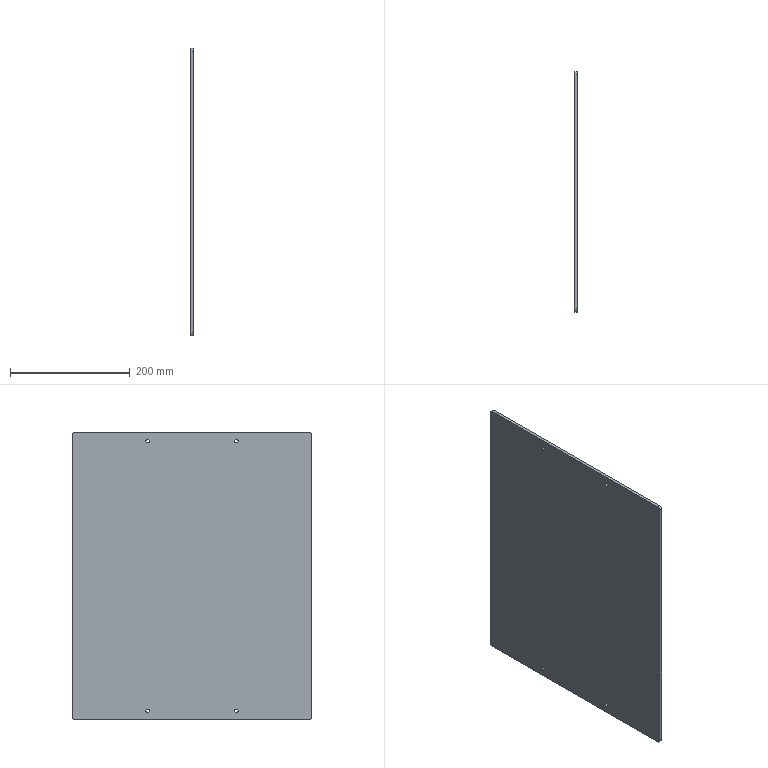Part | SolidWorks | features Extrusion 1, Fillet 1, ICE 1 | 1 solid | 18 faces | box 5 x 400 x 480 mm | volume 959327 mm3 | cylinder 12 | plane 6 | commonest cylinder face diameters 6 x8 10 x4
STEP:
#1=CARTESIAN_POINT('',(0.,-74.,-222.));
#2=VERTEX_POINT('',#1);
#3=CARTESIAN_POINT('',(0.,-74.,-228.));
#4=VERTEX_POINT('',#3);
#5=CARTESIAN_POINT('',(0.,-74.,-225.));
#6=DIRECTION('',(1.,0.,0.));
#7=DIRECTION('',(0.,0.,-1.));
#8=AXIS2_PLACEMENT_3D('',#5,#6,#7);
#9=CIRCLE('',#8,3.);
#10=EDGE_CURVE('',#2,#4,#9,.T.);
#11=ORIENTED_EDGE('',*,*,#10,.F.);
#12=CARTESIAN_POINT('',(5.,-74.,-222.));
#13=VERTEX_POINT('',#12);
#14=CARTESIAN_POINT('',(0.,-74.,-222.));
#15=DIRECTION('',(1.,0.,0.));
#16=VECTOR('',#15,1000.);
#17=LINE('',#14,#16);
#18=EDGE_CURVE('',#2,#13,#17,.T.);
#19=ORIENTED_EDGE('',*,*,#18,.T.);
#20=CARTESIAN_POINT('',(5.,-74.,-228.));
#21=VERTEX_POINT('',#20);
#22=CARTESIAN_POINT('',(5.,-74.,-225.));
#23=DIRECTION('',(1.,0.,0.));
#24=DIRECTION('',(0.,0.,-1.));
#25=AXIS2_PLACEMENT_3D('',#22,#23,#24);
#26=CIRCLE('',#25,3.);
#27=EDGE_CURVE('',#13,#21,#26,.T.);
#28=ORIENTED_EDGE('',*,*,#27,.T.);
#29=CARTESIAN_POINT('',(0.,-74.,-228.));
#30=DIRECTION('',(1.,0.,0.));
#31=VECTOR('',#30,1000.);
#32=LINE('',#29,#31);
#33=EDGE_CURVE('',#4,#21,#32,.T.);
#34=ORIENTED_EDGE('',*,*,#33,.F.);
#35=EDGE_LOOP('',(#11,#19,#28,#34));
#36=FACE_OUTER_BOUND('',#35,.T.);
#37=CARTESIAN_POINT('',(0.,-74.,-225.));
#38=DIRECTION('',(1.,0.,0.));
#39=DIRECTION('',(0.,0.,-1.));
#40=AXIS2_PLACEMENT_3D('',#37,#38,#39);
#41=CYLINDRICAL_SURFACE('',#40,3.);
#42=ADVANCED_FACE('',(#36),#41,.F.);
#43=CARTESIAN_POINT('',(0.,-74.,228.));
#44=VERTEX_POINT('',#43);
#45=CARTESIAN_POINT('',(0.,-74.,222.));
#46=VERTEX_POINT('',#45);
#47=CARTESIAN_POINT('',(0.,-74.,225.));
#48=DIRECTION('',(1.,0.,0.));
#49=DIRECTION('',(0.,0.,-1.));
#50=AXIS2_PLACEMENT_3D('',#47,#48,#49);
#51=CIRCLE('',#50,3.);
#52=EDGE_CURVE('',#44,#46,#51,.T.);
#53=ORIENTED_EDGE('',*,*,#52,.F.);
#54=CARTESIAN_POINT('',(5.,-74.,228.));
#55=VERTEX_POINT('',#54);
#56=CARTESIAN_POINT('',(0.,-74.,228.));
#57=DIRECTION('',(1.,0.,0.));
#58=VECTOR('',#57,1000.);
#59=LINE('',#56,#58);
#60=EDGE_CURVE('',#44,#55,#59,.T.);
#61=ORIENTED_EDGE('',*,*,#60,.T.);
#62=CARTESIAN_POINT('',(5.,-74.,222.));
#63=VERTEX_POINT('',#62);
#64=CARTESIAN_POINT('',(5.,-74.,225.));
#65=DIRECTION('',(1.,0.,0.));
#66=DIRECTION('',(0.,0.,-1.));
#67=AXIS2_PLACEMENT_3D('',#64,#65,#66);
#68=CIRCLE('',#67,3.);
#69=EDGE_CURVE('',#55,#63,#68,.T.);
#70=ORIENTED_EDGE('',*,*,#69,.T.);
#71=CARTESIAN_POINT('',(0.,-74.,222.));
#72=DIRECTION('',(1.,0.,0.));
#73=VECTOR('',#72,1000.);
#74=LINE('',#71,#73);
#75=EDGE_CURVE('',#46,#63,#74,.T.);
#76=ORIENTED_EDGE('',*,*,#75,.F.);
#77=EDGE_LOOP('',(#53,#61,#70,#76));
#78=FACE_OUTER_BOUND('',#77,.T.);
#79=CARTESIAN_POINT('',(0.,-74.,225.));
#80=DIRECTION('',(1.,0.,0.));
#81=DIRECTION('',(0.,0.,-1.));
#82=AXIS2_PLACEMENT_3D('',#79,#80,#81);
#83=CYLINDRICAL_SURFACE('',#82,3.);
#84=ADVANCED_FACE('',(#78),#83,.F.);
#85=CARTESIAN_POINT('',(0.,74.,-222.));
#86=VERTEX_POINT('',#85);
#87=CARTESIAN_POINT('',(0.,74.,-228.));
#88=VERTEX_POINT('',#87);
#89=CARTESIAN_POINT('',(0.,74.,-225.));
#90=DIRECTION('',(1.,0.,0.));
#91=DIRECTION('',(0.,0.,-1.));
#92=AXIS2_PLACEMENT_3D('',#89,#90,#91);
#93=CIRCLE('',#92,3.);
#94=EDGE_CURVE('',#86,#88,#93,.T.);
#95=ORIENTED_EDGE('',*,*,#94,.F.);
#96=CARTESIAN_POINT('',(5.,74.,-222.));
#97=VERTEX_POINT('',#96);
#98=CARTESIAN_POINT('',(0.,74.,-222.));
#99=DIRECTION('',(1.,0.,0.));
#100=VECTOR('',#99,1000.);
#101=LINE('',#98,#100);
#102=EDGE_CURVE('',#86,#97,#101,.T.);
#103=ORIENTED_EDGE('',*,*,#102,.T.);
#104=CARTESIAN_POINT('',(5.,74.,-228.));
#105=VERTEX_POINT('',#104);
#106=CARTESIAN_POINT('',(5.,74.,-225.));
#107=DIRECTION('',(1.,0.,0.));
#108=DIRECTION('',(0.,0.,-1.));
#109=AXIS2_PLACEMENT_3D('',#106,#107,#108);
#110=CIRCLE('',#109,3.);
#111=EDGE_CURVE('',#97,#105,#110,.T.);
#112=ORIENTED_EDGE('',*,*,#111,.T.);
#113=CARTESIAN_POINT('',(0.,74.,-228.));
#114=DIRECTION('',(1.,0.,0.));
#115=VECTOR('',#114,1000.);
#116=LINE('',#113,#115);
#117=EDGE_CURVE('',#88,#105,#116,.T.);
#118=ORIENTED_EDGE('',*,*,#117,.F.);
#119=EDGE_LOOP('',(#95,#103,#112,#118));
#120=FACE_OUTER_BOUND('',#119,.T.);
#121=CARTESIAN_POINT('',(0.,74.,-225.));
#122=DIRECTION('',(1.,0.,0.));
#123=DIRECTION('',(0.,0.,-1.));
#124=AXIS2_PLACEMENT_3D('',#121,#122,#123);
#125=CYLINDRICAL_SURFACE('',#124,3.);
#126=ADVANCED_FACE('',(#120),#125,.F.);
#127=CARTESIAN_POINT('',(0.,74.,228.));
#128=VERTEX_POINT('',#127);
#129=CARTESIAN_POINT('',(0.,74.,222.));
#130=VERTEX_POINT('',#129);
#131=CARTESIAN_POINT('',(0.,74.,225.));
#132=DIRECTION('',(1.,0.,0.));
#133=DIRECTION('',(0.,0.,-1.));
#134=AXIS2_PLACEMENT_3D('',#131,#132,#133);
#135=CIRCLE('',#134,3.);
#136=EDGE_CURVE('',#128,#130,#135,.T.);
#137=ORIENTED_EDGE('',*,*,#136,.F.);
#138=CARTESIAN_POINT('',(5.,74.,228.));
#139=VERTEX_POINT('',#138);
#140=CARTESIAN_POINT('',(0.,74.,228.));
#141=DIRECTION('',(1.,0.,0.));
#142=VECTOR('',#141,1000.);
#143=LINE('',#140,#142);
#144=EDGE_CURVE('',#128,#139,#143,.T.);
#145=ORIENTED_EDGE('',*,*,#144,.T.);
#146=CARTESIAN_POINT('',(5.,74.,222.));
#147=VERTEX_POINT('',#146);
#148=CARTESIAN_POINT('',(5.,74.,225.));
#149=DIRECTION('',(1.,0.,0.));
#150=DIRECTION('',(0.,0.,-1.));
#151=AXIS2_PLACEMENT_3D('',#148,#149,#150);
#152=CIRCLE('',#151,3.);
#153=EDGE_CURVE('',#139,#147,#152,.T.);
#154=ORIENTED_EDGE('',*,*,#153,.T.);
#155=CARTESIAN_POINT('',(0.,74.,222.));
#156=DIRECTION('',(1.,0.,0.));
#157=VECTOR('',#156,1000.);
#158=LINE('',#155,#157);
#159=EDGE_CURVE('',#130,#147,#158,.T.);
#160=ORIENTED_EDGE('',*,*,#159,.F.);
#161=EDGE_LOOP('',(#137,#145,#154,#160));
#162=FACE_OUTER_BOUND('',#161,.T.);
#163=CARTESIAN_POINT('',(0.,74.,225.));
#164=DIRECTION('',(1.,0.,0.));
#165=DIRECTION('',(0.,0.,-1.));
#166=AXIS2_PLACEMENT_3D('',#163,#164,#165);
#167=CYLINDRICAL_SURFACE('',#166,3.);
#168=ADVANCED_FACE('',(#162),#167,.F.);
#169=CARTESIAN_POINT('',(0.,195.,240.));
#170=VERTEX_POINT('',#169);
#171=CARTESIAN_POINT('',(0.,-195.,240.));
#172=VERTEX_POINT('',#171);
#173=CARTESIAN_POINT('',(0.,200.,240.));
#174=DIRECTION('',(0.,-1.,0.));
#175=VECTOR('',#174,1000.);
#176=LINE('',#173,#175);
#177=EDGE_CURVE('',#170,#172,#176,.T.);
#178=ORIENTED_EDGE('',*,*,#177,.T.);
#179=CARTESIAN_POINT('',(5.,-195.,240.));
#180=VERTEX_POINT('',#179);
#181=CARTESIAN_POINT('',(5.,-195.,240.));
#182=DIRECTION('',(1.,0.,0.));
#183=VECTOR('',#182,1000.);
#184=LINE('',#181,#183);
#185=EDGE_CURVE('',#172,#180,#184,.T.);
#186=ORIENTED_EDGE('',*,*,#185,.T.);
#187=CARTESIAN_POINT('',(5.,195.,240.));
#188=VERTEX_POINT('',#187);
#189=CARTESIAN_POINT('',(5.,200.,240.));
#190=DIRECTION('',(0.,-1.,0.));
#191=VECTOR('',#190,1000.);
#192=LINE('',#189,#191);
#193=EDGE_CURVE('',#188,#180,#192,.T.);
#194=ORIENTED_EDGE('',*,*,#193,.F.);
#195=CARTESIAN_POINT('',(5.,195.,240.));
#196=DIRECTION('',(-1.,0.,0.));
#197=VECTOR('',#196,1000.);
#198=LINE('',#195,#197);
#199=EDGE_CURVE('',#188,#170,#198,.T.);
#200=ORIENTED_EDGE('',*,*,#199,.T.);
#201=EDGE_LOOP('',(#178,#186,#194,#200));
#202=FACE_OUTER_BOUND('',#201,.T.);
#203=CARTESIAN_POINT('',(5.,200.,240.));
#204=DIRECTION('',(0.,0.,-1.));
#205=DIRECTION('',(-1.,0.,0.));
#206=AXIS2_PLACEMENT_3D('',#203,#204,#205);
#207=PLANE('',#206);
#208=ADVANCED_FACE('',(#202),#207,.F.);
#209=CARTESIAN_POINT('',(5.,-200.,235.));
#210=VERTEX_POINT('',#209);
#211=CARTESIAN_POINT('',(5.,-200.,-235.));
#212=VERTEX_POINT('',#211);
#213=CARTESIAN_POINT('',(5.,-200.,240.));
#214=DIRECTION('',(0.,0.,-1.));
#215=VECTOR('',#214,1000.);
#216=LINE('',#213,#215);
#217=EDGE_CURVE('',#210,#212,#216,.T.);
#218=ORIENTED_EDGE('',*,*,#217,.F.);
#219=CARTESIAN_POINT('',(0.,-200.,235.));
#220=VERTEX_POINT('',#219);
#221=CARTESIAN_POINT('',(5.,-200.,235.));
#222=DIRECTION('',(-1.,0.,0.));
#223=VECTOR('',#222,1000.);
#224=LINE('',#221,#223);
#225=EDGE_CURVE('',#210,#220,#224,.T.);
#226=ORIENTED_EDGE('',*,*,#225,.T.);
#227=CARTESIAN_POINT('',(0.,-200.,-235.));
#228=VERTEX_POINT('',#227);
#229=CARTESIAN_POINT('',(0.,-200.,240.));
#230=DIRECTION('',(0.,0.,-1.));
#231=VECTOR('',#230,1000.);
#232=LINE('',#229,#231);
#233=EDGE_CURVE('',#220,#228,#232,.T.);
#234=ORIENTED_EDGE('',*,*,#233,.T.);
#235=CARTESIAN_POINT('',(5.,-200.,-235.));
#236=DIRECTION('',(1.,0.,0.));
#237=VECTOR('',#236,1000.);
#238=LINE('',#235,#237);
#239=EDGE_CURVE('',#228,#212,#238,.T.);
#240=ORIENTED_EDGE('',*,*,#239,.T.);
#241=EDGE_LOOP('',(#218,#226,#234,#240));
#242=FACE_OUTER_BOUND('',#241,.T.);
#243=CARTESIAN_POINT('',(5.,-200.,240.));
#244=DIRECTION('',(0.,1.,0.));
#245=DIRECTION('',(0.,0.,1.));
#246=AXIS2_PLACEMENT_3D('',#243,#244,#245);
#247=PLANE('',#246);
#248=ADVANCED_FACE('',(#242),#247,.F.);
#249=CARTESIAN_POINT('',(5.,-195.,-240.));
#250=VERTEX_POINT('',#249);
#251=CARTESIAN_POINT('',(5.,195.,-240.));
#252=VERTEX_POINT('',#251);
#253=CARTESIAN_POINT('',(5.,200.,-240.));
#254=DIRECTION('',(0.,1.,0.));
#255=VECTOR('',#254,1000.);
#256=LINE('',#253,#255);
#257=EDGE_CURVE('',#250,#252,#256,.T.);
#258=ORIENTED_EDGE('',*,*,#257,.F.);
#259=CARTESIAN_POINT('',(0.,-195.,-240.));
#260=VERTEX_POINT('',#259);
#261=CARTESIAN_POINT('',(5.,-195.,-240.));
#262=DIRECTION('',(-1.,0.,0.));
#263=VECTOR('',#262,1000.);
#264=LINE('',#261,#263);
#265=EDGE_CURVE('',#250,#260,#264,.T.);
#266=ORIENTED_EDGE('',*,*,#265,.T.);
#267=CARTESIAN_POINT('',(0.,195.,-240.));
#268=VERTEX_POINT('',#267);
#269=CARTESIAN_POINT('',(0.,200.,-240.));
#270=DIRECTION('',(0.,1.,0.));
#271=VECTOR('',#270,1000.);
#272=LINE('',#269,#271);
#273=EDGE_CURVE('',#260,#268,#272,.T.);
#274=ORIENTED_EDGE('',*,*,#273,.T.);
#275=CARTESIAN_POINT('',(5.,195.,-240.));
#276=DIRECTION('',(1.,0.,0.));
#277=VECTOR('',#276,1000.);
#278=LINE('',#275,#277);
#279=EDGE_CURVE('',#268,#252,#278,.T.);
#280=ORIENTED_EDGE('',*,*,#279,.T.);
#281=EDGE_LOOP('',(#258,#266,#274,#280));
#282=FACE_OUTER_BOUND('',#281,.T.);
#283=CARTESIAN_POINT('',(5.,200.,-240.));
#284=DIRECTION('',(0.,0.,1.));
#285=DIRECTION('',(1.,0.,0.));
#286=AXIS2_PLACEMENT_3D('',#283,#284,#285);
#287=PLANE('',#286);
#288=ADVANCED_FACE('',(#282),#287,.F.);
#289=CARTESIAN_POINT('',(5.,200.,-235.));
#290=VERTEX_POINT('',#289);
#291=CARTESIAN_POINT('',(5.,200.,235.));
#292=VERTEX_POINT('',#291);
#293=CARTESIAN_POINT('',(5.,200.,240.));
#294=DIRECTION('',(0.,0.,1.));
#295=VECTOR('',#294,1000.);
#296=LINE('',#293,#295);
#297=EDGE_CURVE('',#290,#292,#296,.T.);
#298=ORIENTED_EDGE('',*,*,#297,.F.);
#299=CARTESIAN_POINT('',(0.,200.,-235.));
#300=VERTEX_POINT('',#299);
#301=CARTESIAN_POINT('',(5.,200.,-235.));
#302=DIRECTION('',(-1.,0.,0.));
#303=VECTOR('',#302,1000.);
#304=LINE('',#301,#303);
#305=EDGE_CURVE('',#290,#300,#304,.T.);
#306=ORIENTED_EDGE('',*,*,#305,.T.);
#307=CARTESIAN_POINT('',(0.,200.,235.));
#308=VERTEX_POINT('',#307);
#309=CARTESIAN_POINT('',(0.,200.,240.));
#310=DIRECTION('',(0.,0.,1.));
#311=VECTOR('',#310,1000.);
#312=LINE('',#309,#311);
#313=EDGE_CURVE('',#300,#308,#312,.T.);
#314=ORIENTED_EDGE('',*,*,#313,.T.);
#315=CARTESIAN_POINT('',(5.,200.,235.));
#316=DIRECTION('',(1.,0.,0.));
#317=VECTOR('',#316,1000.);
#318=LINE('',#315,#317);
#319=EDGE_CURVE('',#308,#292,#318,.T.);
#320=ORIENTED_EDGE('',*,*,#319,.T.);
#321=EDGE_LOOP('',(#298,#306,#314,#320));
#322=FACE_OUTER_BOUND('',#321,.T.);
#323=CARTESIAN_POINT('',(5.,200.,240.));
#324=DIRECTION('',(0.,-1.,0.));
#325=DIRECTION('',(0.,0.,-1.));
#326=AXIS2_PLACEMENT_3D('',#323,#324,#325);
#327=PLANE('',#326);
#328=ADVANCED_FACE('',(#322),#327,.F.);
#329=CARTESIAN_POINT('',(5.,-74.,-225.));
#330=DIRECTION('',(1.,0.,0.));
#331=DIRECTION('',(0.,0.,-1.));
#332=AXIS2_PLACEMENT_3D('',#329,#330,#331);
#333=CIRCLE('',#332,3.);
#334=EDGE_CURVE('',#21,#13,#333,.T.);
#335=ORIENTED_EDGE('',*,*,#334,.F.);
#336=ORIENTED_EDGE('',*,*,#27,.F.);
#337=EDGE_LOOP('',(#335,#336));
#338=FACE_BOUND('',#337,.T.);
#339=CARTESIAN_POINT('',(5.,-74.,225.));
#340=DIRECTION('',(1.,0.,0.));
#341=DIRECTION('',(0.,0.,-1.));
#342=AXIS2_PLACEMENT_3D('',#339,#340,#341);
#343=CIRCLE('',#342,3.);
#344=EDGE_CURVE('',#63,#55,#343,.T.);
#345=ORIENTED_EDGE('',*,*,#344,.F.);
#346=ORIENTED_EDGE('',*,*,#69,.F.);
#347=EDGE_LOOP('',(#345,#346));
#348=FACE_BOUND('',#347,.T.);
#349=CARTESIAN_POINT('',(5.,74.,-225.));
#350=DIRECTION('',(1.,0.,0.));
#351=DIRECTION('',(0.,0.,-1.));
#352=AXIS2_PLACEMENT_3D('',#349,#350,#351);
#353=CIRCLE('',#352,3.);
#354=EDGE_CURVE('',#105,#97,#353,.T.);
#355=ORIENTED_EDGE('',*,*,#354,.F.);
#356=ORIENTED_EDGE('',*,*,#111,.F.);
#357=EDGE_LOOP('',(#355,#356));
#358=FACE_BOUND('',#357,.T.);
#359=CARTESIAN_POINT('',(5.,74.,225.));
#360=DIRECTION('',(1.,0.,0.));
#361=DIRECTION('',(0.,0.,-1.));
#362=AXIS2_PLACEMENT_3D('',#359,#360,#361);
#363=CIRCLE('',#362,3.);
#364=EDGE_CURVE('',#147,#139,#363,.T.);
#365=ORIENTED_EDGE('',*,*,#364,.F.);
#366=ORIENTED_EDGE('',*,*,#153,.F.);
#367=EDGE_LOOP('',(#365,#366));
#368=FACE_BOUND('',#367,.T.);
#369=ORIENTED_EDGE('',*,*,#193,.T.);
#370=CARTESIAN_POINT('',(5.,-195.,235.));
#371=DIRECTION('',(1.,0.,0.));
#372=DIRECTION('',(0.,0.,-1.));
#373=AXIS2_PLACEMENT_3D('',#370,#371,#372);
#374=CIRCLE('',#373,5.);
#375=EDGE_CURVE('',#180,#210,#374,.T.);
#376=ORIENTED_EDGE('',*,*,#375,.T.);
#377=ORIENTED_EDGE('',*,*,#217,.T.);
#378=CARTESIAN_POINT('',(5.,-195.,-235.));
#379=DIRECTION('',(1.,0.,0.));
#380=DIRECTION('',(0.,0.,-1.));
#381=AXIS2_PLACEMENT_3D('',#378,#379,#380);
#382=CIRCLE('',#381,5.);
#383=EDGE_CURVE('',#212,#250,#382,.T.);
#384=ORIENTED_EDGE('',*,*,#383,.T.);
#385=ORIENTED_EDGE('',*,*,#257,.T.);
#386=CARTESIAN_POINT('',(5.,195.,-235.));
#387=DIRECTION('',(1.,0.,0.));
#388=DIRECTION('',(0.,0.,-1.));
#389=AXIS2_PLACEMENT_3D('',#386,#387,#388);
#390=CIRCLE('',#389,5.);
#391=EDGE_CURVE('',#252,#290,#390,.T.);
#392=ORIENTED_EDGE('',*,*,#391,.T.);
#393=ORIENTED_EDGE('',*,*,#297,.T.);
#394=CARTESIAN_POINT('',(5.,195.,235.));
#395=DIRECTION('',(1.,0.,0.));
#396=DIRECTION('',(0.,0.,-1.));
#397=AXIS2_PLACEMENT_3D('',#394,#395,#396);
#398=CIRCLE('',#397,5.);
#399=EDGE_CURVE('',#292,#188,#398,.T.);
#400=ORIENTED_EDGE('',*,*,#399,.T.);
#401=EDGE_LOOP('',(#369,#376,#377,#384,#385,#392,#393,#400));
#402=FACE_OUTER_BOUND('',#401,.T.);
#403=CARTESIAN_POINT('',(5.,0.,0.));
#404=DIRECTION('',(1.,0.,0.));
#405=DIRECTION('',(0.,0.,-1.));
#406=AXIS2_PLACEMENT_3D('',#403,#404,#405);
#407=PLANE('',#406);
#408=ADVANCED_FACE('',(#338,#348,#358,#368,#402),#407,.T.);
#409=CARTESIAN_POINT('',(0.,-74.,-225.));
#410=DIRECTION('',(1.,0.,0.));
#411=DIRECTION('',(0.,0.,-1.));
#412=AXIS2_PLACEMENT_3D('',#409,#410,#411);
#413=CIRCLE('',#412,3.);
#414=EDGE_CURVE('',#4,#2,#413,.T.);
#415=ORIENTED_EDGE('',*,*,#414,.T.);
#416=ORIENTED_EDGE('',*,*,#10,.T.);
#417=EDGE_LOOP('',(#415,#416));
#418=FACE_BOUND('',#417,.T.);
#419=CARTESIAN_POINT('',(0.,-74.,225.));
#420=DIRECTION('',(1.,0.,0.));
#421=DIRECTION('',(0.,0.,-1.));
#422=AXIS2_PLACEMENT_3D('',#419,#420,#421);
#423=CIRCLE('',#422,3.);
#424=EDGE_CURVE('',#46,#44,#423,.T.);
#425=ORIENTED_EDGE('',*,*,#424,.T.);
#426=ORIENTED_EDGE('',*,*,#52,.T.);
#427=EDGE_LOOP('',(#425,#426));
#428=FACE_BOUND('',#427,.T.);
#429=CARTESIAN_POINT('',(0.,74.,-225.));
#430=DIRECTION('',(1.,0.,0.));
#431=DIRECTION('',(0.,0.,-1.));
#432=AXIS2_PLACEMENT_3D('',#429,#430,#431);
#433=CIRCLE('',#432,3.);
#434=EDGE_CURVE('',#88,#86,#433,.T.);
#435=ORIENTED_EDGE('',*,*,#434,.T.);
#436=ORIENTED_EDGE('',*,*,#94,.T.);
#437=EDGE_LOOP('',(#435,#436));
#438=FACE_BOUND('',#437,.T.);
#439=CARTESIAN_POINT('',(0.,74.,225.));
#440=DIRECTION('',(1.,0.,0.));
#441=DIRECTION('',(0.,0.,-1.));
#442=AXIS2_PLACEMENT_3D('',#439,#440,#441);
#443=CIRCLE('',#442,3.);
#444=EDGE_CURVE('',#130,#128,#443,.T.);
#445=ORIENTED_EDGE('',*,*,#444,.T.);
#446=ORIENTED_EDGE('',*,*,#136,.T.);
#447=EDGE_LOOP('',(#445,#446));
#448=FACE_BOUND('',#447,.T.);
#449=ORIENTED_EDGE('',*,*,#233,.F.);
#450=CARTESIAN_POINT('',(0.,-195.,235.));
#451=DIRECTION('',(-1.,0.,0.));
#452=DIRECTION('',(0.,0.,-1.));
#453=AXIS2_PLACEMENT_3D('',#450,#451,#452);
#454=CIRCLE('',#453,5.);
#455=EDGE_CURVE('',#220,#172,#454,.T.);
#456=ORIENTED_EDGE('',*,*,#455,.T.);
#457=ORIENTED_EDGE('',*,*,#177,.F.);
#458=CARTESIAN_POINT('',(0.,195.,235.));
#459=DIRECTION('',(-1.,0.,0.));
#460=DIRECTION('',(0.,0.,-1.));
#461=AXIS2_PLACEMENT_3D('',#458,#459,#460);
#462=CIRCLE('',#461,5.);
#463=EDGE_CURVE('',#170,#308,#462,.T.);
#464=ORIENTED_EDGE('',*,*,#463,.T.);
#465=ORIENTED_EDGE('',*,*,#313,.F.);
#466=CARTESIAN_POINT('',(0.,195.,-235.));
#467=DIRECTION('',(-1.,0.,0.));
#468=DIRECTION('',(0.,0.,-1.));
#469=AXIS2_PLACEMENT_3D('',#466,#467,#468);
#470=CIRCLE('',#469,5.);
#471=EDGE_CURVE('',#300,#268,#470,.T.);
#472=ORIENTED_EDGE('',*,*,#471,.T.);
#473=ORIENTED_EDGE('',*,*,#273,.F.);
#474=CARTESIAN_POINT('',(0.,-195.,-235.));
#475=DIRECTION('',(-1.,0.,0.));
#476=DIRECTION('',(0.,0.,-1.));
#477=AXIS2_PLACEMENT_3D('',#474,#475,#476);
#478=CIRCLE('',#477,5.);
#479=EDGE_CURVE('',#260,#228,#478,.T.);
#480=ORIENTED_EDGE('',*,*,#479,.T.);
#481=EDGE_LOOP('',(#449,#456,#457,#464,#465,#472,#473,#480));
#482=FACE_OUTER_BOUND('',#481,.T.);
#483=CARTESIAN_POINT('',(0.,0.,0.));
#484=DIRECTION('',(1.,0.,0.));
#485=DIRECTION('',(0.,0.,-1.));
#486=AXIS2_PLACEMENT_3D('',#483,#484,#485);
#487=PLANE('',#486);
#488=ADVANCED_FACE('',(#418,#428,#438,#448,#482),#487,.F.);
#489=ORIENTED_EDGE('',*,*,#144,.F.);
#490=ORIENTED_EDGE('',*,*,#444,.F.);
#491=ORIENTED_EDGE('',*,*,#159,.T.);
#492=ORIENTED_EDGE('',*,*,#364,.T.);
#493=EDGE_LOOP('',(#489,#490,#491,#492));
#494=FACE_OUTER_BOUND('',#493,.T.);
#495=CARTESIAN_POINT('',(0.,74.,225.));
#496=DIRECTION('',(1.,0.,0.));
#497=DIRECTION('',(0.,0.,-1.));
#498=AXIS2_PLACEMENT_3D('',#495,#496,#497);
#499=CYLINDRICAL_SURFACE('',#498,3.);
#500=ADVANCED_FACE('',(#494),#499,.F.);
#501=ORIENTED_EDGE('',*,*,#102,.F.);
#502=ORIENTED_EDGE('',*,*,#434,.F.);
#503=ORIENTED_EDGE('',*,*,#117,.T.);
#504=ORIENTED_EDGE('',*,*,#354,.T.);
#505=EDGE_LOOP('',(#501,#502,#503,#504));
#506=FACE_OUTER_BOUND('',#505,.T.);
#507=CARTESIAN_POINT('',(0.,74.,-225.));
#508=DIRECTION('',(1.,0.,0.));
#509=DIRECTION('',(0.,0.,-1.));
#510=AXIS2_PLACEMENT_3D('',#507,#508,#509);
#511=CYLINDRICAL_SURFACE('',#510,3.);
#512=ADVANCED_FACE('',(#506),#511,.F.);
#513=ORIENTED_EDGE('',*,*,#60,.F.);
#514=ORIENTED_EDGE('',*,*,#424,.F.);
#515=ORIENTED_EDGE('',*,*,#75,.T.);
#516=ORIENTED_EDGE('',*,*,#344,.T.);
#517=EDGE_LOOP('',(#513,#514,#515,#516));
#518=FACE_OUTER_BOUND('',#517,.T.);
#519=CARTESIAN_POINT('',(0.,-74.,225.));
#520=DIRECTION('',(1.,0.,0.));
#521=DIRECTION('',(0.,0.,-1.));
#522=AXIS2_PLACEMENT_3D('',#519,#520,#521);
#523=CYLINDRICAL_SURFACE('',#522,3.);
#524=ADVANCED_FACE('',(#518),#523,.F.);
#525=ORIENTED_EDGE('',*,*,#18,.F.);
#526=ORIENTED_EDGE('',*,*,#414,.F.);
#527=ORIENTED_EDGE('',*,*,#33,.T.);
#528=ORIENTED_EDGE('',*,*,#334,.T.);
#529=EDGE_LOOP('',(#525,#526,#527,#528));
#530=FACE_OUTER_BOUND('',#529,.T.);
#531=CARTESIAN_POINT('',(0.,-74.,-225.));
#532=DIRECTION('',(1.,0.,0.));
#533=DIRECTION('',(0.,0.,-1.));
#534=AXIS2_PLACEMENT_3D('',#531,#532,#533);
#535=CYLINDRICAL_SURFACE('',#534,3.);
#536=ADVANCED_FACE('',(#530),#535,.F.);
#537=ORIENTED_EDGE('',*,*,#375,.F.);
#538=ORIENTED_EDGE('',*,*,#185,.F.);
#539=ORIENTED_EDGE('',*,*,#455,.F.);
#540=ORIENTED_EDGE('',*,*,#225,.F.);
#541=EDGE_LOOP('',(#537,#538,#539,#540));
#542=FACE_OUTER_BOUND('',#541,.T.);
#543=CARTESIAN_POINT('',(5.,-195.,235.));
#544=DIRECTION('',(-1.,0.,0.));
#545=DIRECTION('',(0.,0.,1.));
#546=AXIS2_PLACEMENT_3D('',#543,#544,#545);
#547=CYLINDRICAL_SURFACE('',#546,5.);
#548=ADVANCED_FACE('',(#542),#547,.T.);
#549=ORIENTED_EDGE('',*,*,#383,.F.);
#550=ORIENTED_EDGE('',*,*,#239,.F.);
#551=ORIENTED_EDGE('',*,*,#479,.F.);
#552=ORIENTED_EDGE('',*,*,#265,.F.);
#553=EDGE_LOOP('',(#549,#550,#551,#552));
#554=FACE_OUTER_BOUND('',#553,.T.);
#555=CARTESIAN_POINT('',(5.,-195.,-235.));
#556=DIRECTION('',(-1.,0.,0.));
#557=DIRECTION('',(0.,0.,1.));
#558=AXIS2_PLACEMENT_3D('',#555,#556,#557);
#559=CYLINDRICAL_SURFACE('',#558,5.);
#560=ADVANCED_FACE('',(#554),#559,.T.);
#561=ORIENTED_EDGE('',*,*,#391,.F.);
#562=ORIENTED_EDGE('',*,*,#279,.F.);
#563=ORIENTED_EDGE('',*,*,#471,.F.);
#564=ORIENTED_EDGE('',*,*,#305,.F.);
#565=EDGE_LOOP('',(#561,#562,#563,#564));
#566=FACE_OUTER_BOUND('',#565,.T.);
#567=CARTESIAN_POINT('',(5.,195.,-235.));
#568=DIRECTION('',(-1.,0.,0.));
#569=DIRECTION('',(0.,0.,1.));
#570=AXIS2_PLACEMENT_3D('',#567,#568,#569);
#571=CYLINDRICAL_SURFACE('',#570,5.);
#572=ADVANCED_FACE('',(#566),#571,.T.);
#573=ORIENTED_EDGE('',*,*,#399,.F.);
#574=ORIENTED_EDGE('',*,*,#319,.F.);
#575=ORIENTED_EDGE('',*,*,#463,.F.);
#576=ORIENTED_EDGE('',*,*,#199,.F.);
#577=EDGE_LOOP('',(#573,#574,#575,#576));
#578=FACE_OUTER_BOUND('',#577,.T.);
#579=CARTESIAN_POINT('',(5.,195.,235.));
#580=DIRECTION('',(-1.,0.,0.));
#581=DIRECTION('',(0.,0.,1.));
#582=AXIS2_PLACEMENT_3D('',#579,#580,#581);
#583=CYLINDRICAL_SURFACE('',#582,5.);
#584=ADVANCED_FACE('',(#578),#583,.T.);
#585=CLOSED_SHELL('',(#42,#84,#126,#168,#208,#248,#288,#328,#408,#488,#500,#512,#524,#536,#548,#560,#572,#584));
#586=MANIFOLD_SOLID_BREP('',#585);
#587=CARTESIAN_POINT('',(0.,0.,0.));
#588=DIRECTION('',(0.,0.,1.));
#589=DIRECTION('',(1.,0.,0.));
#590=AXIS2_PLACEMENT_3D('',#587,#588,#589);
#591=(LENGTH_UNIT()NAMED_UNIT(*)SI_UNIT(.MILLI.,.METRE.));
#592=UNCERTAINTY_MEASURE_WITH_UNIT(LENGTH_MEASURE(0.00001),#591,'','');
#593=(NAMED_UNIT(*)PLANE_ANGLE_UNIT()SI_UNIT($,.RADIAN.));
#594=(NAMED_UNIT(*)SI_UNIT($,.STERADIAN.)SOLID_ANGLE_UNIT());
#595=(GEOMETRIC_REPRESENTATION_CONTEXT(3)GLOBAL_UNCERTAINTY_ASSIGNED_CONTEXT((#592))GLOBAL_UNIT_ASSIGNED_CONTEXT((#591,#593,#594))REPRESENTATION_CONTEXT('',''));
#596=ADVANCED_BREP_SHAPE_REPRESENTATION('',(#586,#590),#595);